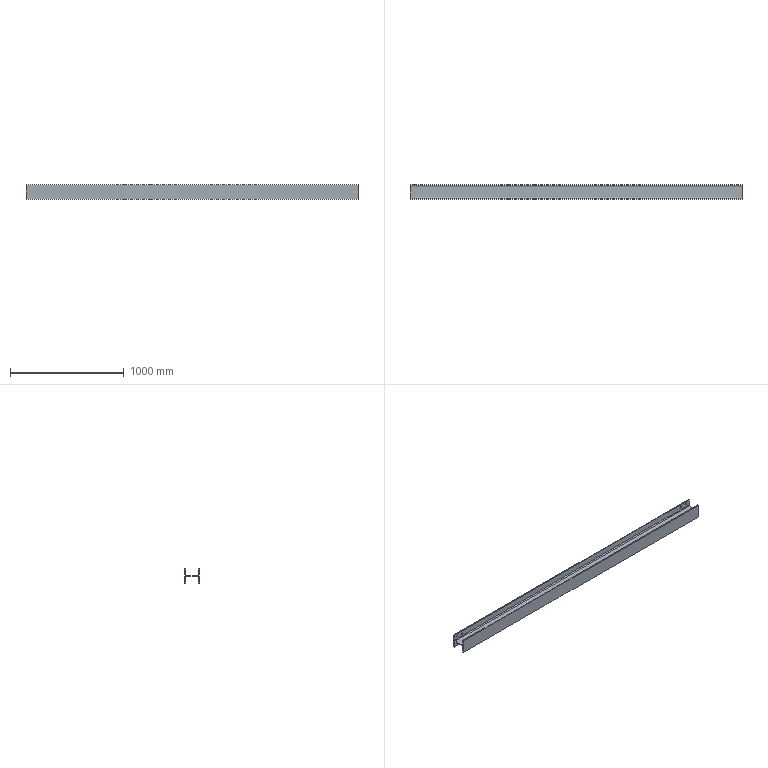Part | STEP file | 04-H125X125X6.5X9_default<machining> | 1 solid | 34 faces | box 2916 x 125 x 125 mm | volume 8741134 mm3 | cylinder 20 | plane 14 | commonest cylinder face diameters 12 x16 16 x4